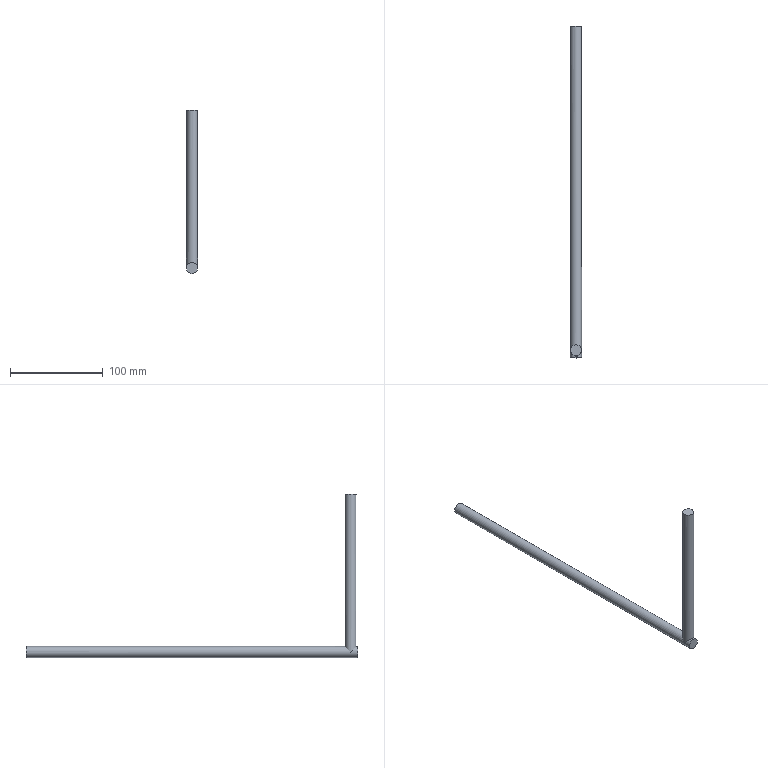Part | STEP file | solid 139 | 1 solid | 5 faces | box 12 x 358 x 176 mm | volume 59139 mm3 | plane 3 | cylinder 2 | commonest cylinder face diameters 12 x2